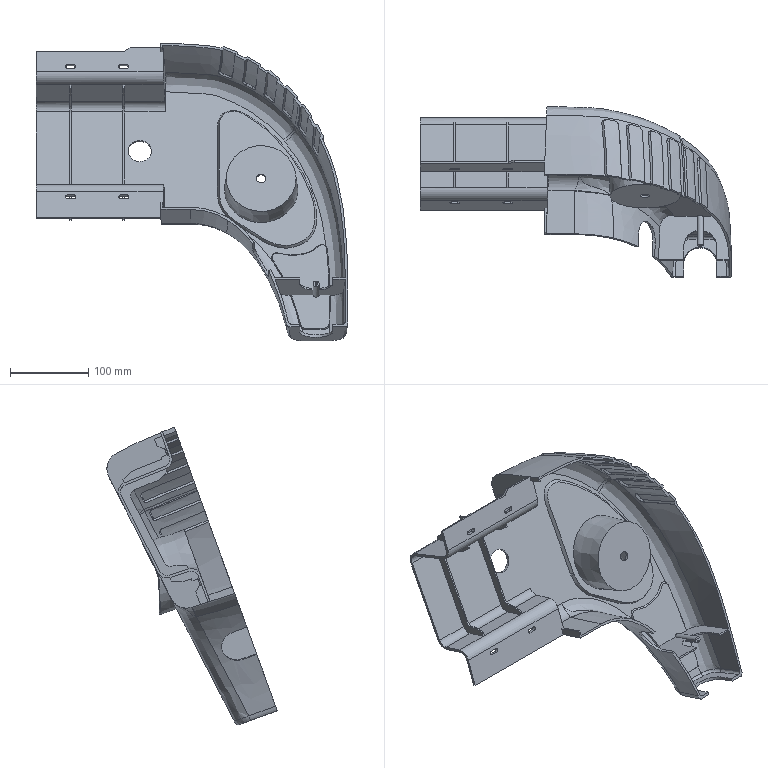Part | STEP file | Consen Cover L | 1 solid | 463 faces | box 398.708 x 218.09 x 381.338 mm | volume 579816 mm3 | plane 216 | spline 156 | cylinder 89 | cone 2 | commonest cylinder face diameters 4.623 x17 4.657 x13 20 x12 5 x8 9 x8 16 x4